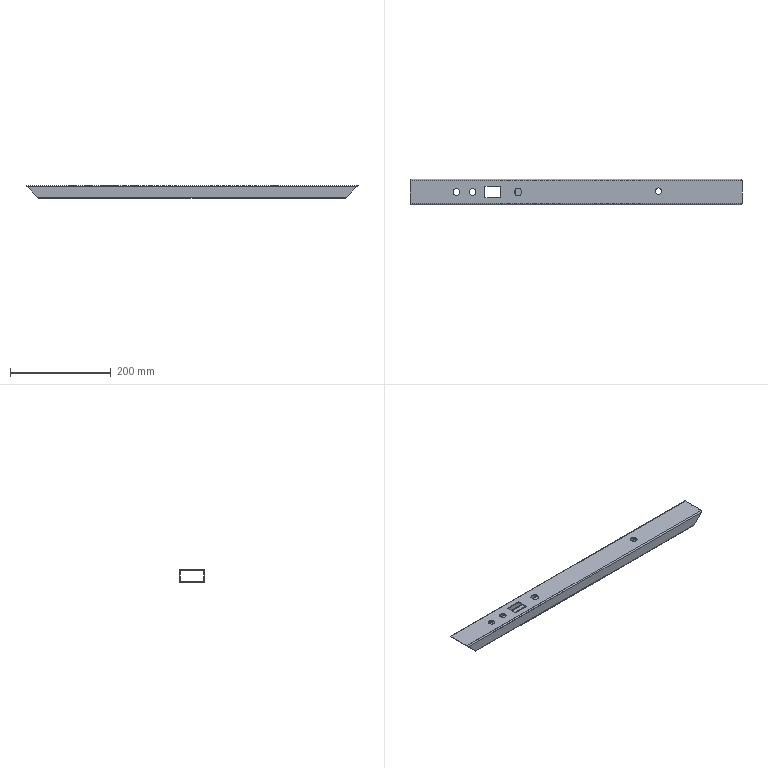Part | STEP file | Q7C0502 | 1 solid | 34 faces | box 658 x 50 x 25 mm | volume 125904 mm3 | plane 20 | cylinder 14 | commonest cylinder face diameters 2 x4 5 x4 13 x4 15.8 x2